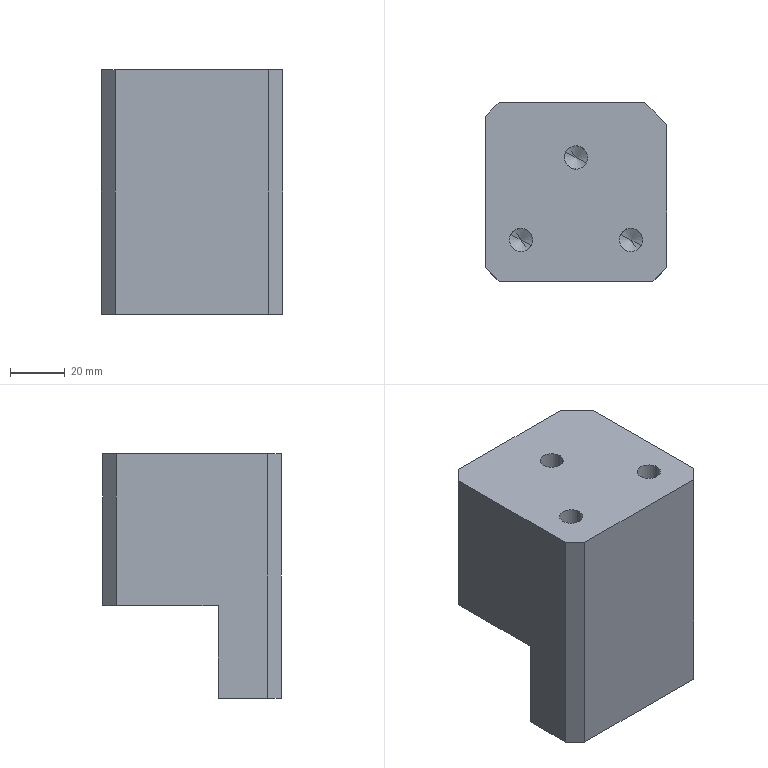Part | CATIA | 1 solid | 40 faces | box 66 x 65 x 89 mm | volume 271119 mm3 | cone 14 | cylinder 14 | plane 12 | commonest cylinder face diameters 8.5 x12 10 x2
STEP:
#1=CARTESIAN_POINT('',(63.,-90.,84.));
#2=VERTEX_POINT('',#1);
#3=CARTESIAN_POINT('',(58.,-85.,84.));
#4=VERTEX_POINT('',#3);
#5=CARTESIAN_POINT('',(60.5,-87.5,84.));
#6=DIRECTION('',(-0.7071,0.7071,0.));
#7=VECTOR('',#6,1.);
#8=LINE('',#5,#7);
#9=EDGE_CURVE('',#2,#4,#8,.T.);
#10=ORIENTED_EDGE('',*,*,#9,.T.);
#11=CARTESIAN_POINT('',(58.,-85.,-5.));
#12=VERTEX_POINT('',#11);
#13=CARTESIAN_POINT('',(58.,-85.,39.5));
#14=DIRECTION('',(0.,0.,1.));
#15=VECTOR('',#14,1.);
#16=LINE('',#13,#15);
#17=EDGE_CURVE('',#12,#4,#16,.T.);
#18=ORIENTED_EDGE('',*,*,#17,.F.);
#19=CARTESIAN_POINT('',(63.,-90.,-5.));
#20=VERTEX_POINT('',#19);
#21=CARTESIAN_POINT('',(60.5,-87.5,-5.));
#22=DIRECTION('',(-0.7071,0.7071,0.));
#23=VECTOR('',#22,1.);
#24=LINE('',#21,#23);
#25=EDGE_CURVE('',#12,#20,#24,.F.);
#26=ORIENTED_EDGE('',*,*,#25,.T.);
#27=CARTESIAN_POINT('',(63.,-90.,39.5));
#28=DIRECTION('',(0.,0.,1.));
#29=VECTOR('',#28,1.);
#30=LINE('',#27,#29);
#31=EDGE_CURVE('',#20,#2,#30,.T.);
#32=ORIENTED_EDGE('',*,*,#31,.T.);
#33=EDGE_LOOP('',(#10,#18,#26,#32));
#34=FACE_OUTER_BOUND('',#33,.T.);
#35=CARTESIAN_POINT('',(63.,-90.,-22.8));
#36=DIRECTION('',(-0.7071,-0.7071,0.));
#37=DIRECTION('',(0.,0.,1.));
#38=AXIS2_PLACEMENT_3D('',#35,#36,#37);
#39=PLANE('',#38);
#40=ADVANCED_FACE('',(#34),#39,.T.);
#41=CARTESIAN_POINT('',(119.,-90.,84.));
#42=VERTEX_POINT('',#41);
#43=CARTESIAN_POINT('',(91.,-90.,84.));
#44=DIRECTION('',(1.,0.,0.));
#45=VECTOR('',#44,1.);
#46=LINE('',#43,#45);
#47=EDGE_CURVE('',#2,#42,#46,.T.);
#48=ORIENTED_EDGE('',*,*,#47,.F.);
#49=ORIENTED_EDGE('',*,*,#31,.F.);
#50=CARTESIAN_POINT('',(119.,-90.,-5.));
#51=VERTEX_POINT('',#50);
#52=CARTESIAN_POINT('',(91.,-90.,-5.));
#53=DIRECTION('',(1.,0.,0.));
#54=VECTOR('',#53,1.);
#55=LINE('',#52,#54);
#56=EDGE_CURVE('',#51,#20,#55,.F.);
#57=ORIENTED_EDGE('',*,*,#56,.F.);
#58=CARTESIAN_POINT('',(119.,-90.,39.5));
#59=DIRECTION('',(0.,0.,-1.));
#60=VECTOR('',#59,1.);
#61=LINE('',#58,#60);
#62=EDGE_CURVE('',#51,#42,#61,.F.);
#63=ORIENTED_EDGE('',*,*,#62,.T.);
#64=EDGE_LOOP('',(#48,#49,#57,#63));
#65=FACE_OUTER_BOUND('',#64,.T.);
#66=CARTESIAN_POINT('',(58.,-90.,0.));
#67=DIRECTION('',(0.,-1.,0.));
#68=DIRECTION('',(1.,0.,0.));
#69=AXIS2_PLACEMENT_3D('',#66,#67,#68);
#70=PLANE('',#69);
#71=ADVANCED_FACE('',(#65),#70,.T.);
#72=CARTESIAN_POINT('',(124.,-85.,84.));
#73=VERTEX_POINT('',#72);
#74=CARTESIAN_POINT('',(121.5,-87.5,84.));
#75=DIRECTION('',(0.7071,0.7071,0.));
#76=VECTOR('',#75,1.);
#77=LINE('',#74,#76);
#78=EDGE_CURVE('',#73,#42,#77,.F.);
#79=ORIENTED_EDGE('',*,*,#78,.T.);
#80=ORIENTED_EDGE('',*,*,#62,.F.);
#81=CARTESIAN_POINT('',(124.,-85.,-5.));
#82=VERTEX_POINT('',#81);
#83=CARTESIAN_POINT('',(121.5,-87.5,-5.));
#84=DIRECTION('',(0.7071,0.7071,0.));
#85=VECTOR('',#84,1.);
#86=LINE('',#83,#85);
#87=EDGE_CURVE('',#51,#82,#86,.T.);
#88=ORIENTED_EDGE('',*,*,#87,.T.);
#89=CARTESIAN_POINT('',(124.,-85.,39.5));
#90=DIRECTION('',(0.,0.,-1.));
#91=VECTOR('',#90,1.);
#92=LINE('',#89,#91);
#93=EDGE_CURVE('',#82,#73,#92,.F.);
#94=ORIENTED_EDGE('',*,*,#93,.T.);
#95=EDGE_LOOP('',(#79,#80,#88,#94));
#96=FACE_OUTER_BOUND('',#95,.T.);
#97=CARTESIAN_POINT('',(119.,-90.,101.8));
#98=DIRECTION('',(0.7071,-0.7071,0.));
#99=DIRECTION('',(0.,0.,-1.));
#100=AXIS2_PLACEMENT_3D('',#97,#98,#99);
#101=PLANE('',#100);
#102=ADVANCED_FACE('',(#96),#101,.T.);
#103=CARTESIAN_POINT('',(116.,-25.,84.));
#104=VERTEX_POINT('',#103);
#105=CARTESIAN_POINT('',(63.,-25.,84.));
#106=VERTEX_POINT('',#105);
#107=CARTESIAN_POINT('',(89.5,-25.,84.));
#108=DIRECTION('',(-1.,0.,0.));
#109=VECTOR('',#108,1.);
#110=LINE('',#107,#109);
#111=EDGE_CURVE('',#104,#106,#110,.T.);
#112=ORIENTED_EDGE('',*,*,#111,.T.);
#113=CARTESIAN_POINT('',(58.,-30.,84.));
#114=VERTEX_POINT('',#113);
#115=CARTESIAN_POINT('',(60.5,-27.5,84.));
#116=DIRECTION('',(0.7071,0.7071,0.));
#117=VECTOR('',#116,1.);
#118=LINE('',#115,#117);
#119=EDGE_CURVE('',#114,#106,#118,.T.);
#120=ORIENTED_EDGE('',*,*,#119,.F.);
#121=CARTESIAN_POINT('',(58.,-57.5,84.));
#122=DIRECTION('',(0.,1.,0.));
#123=VECTOR('',#122,1.);
#124=LINE('',#121,#123);
#125=EDGE_CURVE('',#4,#114,#124,.T.);
#126=ORIENTED_EDGE('',*,*,#125,.F.);
#127=ORIENTED_EDGE('',*,*,#9,.F.);
#128=ORIENTED_EDGE('',*,*,#47,.T.);
#129=ORIENTED_EDGE('',*,*,#78,.F.);
#130=CARTESIAN_POINT('',(124.,-33.,84.));
#131=VERTEX_POINT('',#130);
#132=CARTESIAN_POINT('',(124.,-59.,84.));
#133=DIRECTION('',(0.,-1.,0.));
#134=VECTOR('',#133,1.);
#135=LINE('',#132,#134);
#136=EDGE_CURVE('',#131,#73,#135,.T.);
#137=ORIENTED_EDGE('',*,*,#136,.F.);
#138=CARTESIAN_POINT('',(120.,-29.,84.));
#139=DIRECTION('',(0.7071,-0.7071,0.));
#140=VECTOR('',#139,1.);
#141=LINE('',#138,#140);
#142=EDGE_CURVE('',#104,#131,#141,.T.);
#143=ORIENTED_EDGE('',*,*,#142,.F.);
#144=EDGE_LOOP('',(#112,#120,#126,#127,#128,#129,#137,#143));
#145=FACE_OUTER_BOUND('',#144,.T.);
#146=CARTESIAN_POINT('',(114.73,-77.038,84.));
#147=VERTEX_POINT('',#146);
#148=CARTESIAN_POINT('',(107.27,-72.962,84.));
#149=VERTEX_POINT('',#148);
#150=CARTESIAN_POINT('',(111.,-75.,84.));
#151=DIRECTION('',(0.,0.,1.));
#152=AXIS2_PLACEMENT_3D('',#150,#151,$);
#153=CIRCLE('',#152,4.25);
#154=EDGE_CURVE('',#147,#149,#153,.T.);
#155=ORIENTED_EDGE('',*,*,#154,.F.);
#156=CARTESIAN_POINT('',(111.,-75.,84.));
#157=DIRECTION('',(0.,0.,1.));
#158=AXIS2_PLACEMENT_3D('',#156,#157,$);
#159=CIRCLE('',#158,4.25);
#160=EDGE_CURVE('',#149,#147,#159,.T.);
#161=ORIENTED_EDGE('',*,*,#160,.F.);
#162=EDGE_LOOP('',(#155,#161));
#163=FACE_BOUND('',#162,.T.);
#164=CARTESIAN_POINT('',(74.73,-77.038,84.));
#165=VERTEX_POINT('',#164);
#166=CARTESIAN_POINT('',(67.27,-72.962,84.));
#167=VERTEX_POINT('',#166);
#168=CARTESIAN_POINT('',(71.,-75.,84.));
#169=DIRECTION('',(0.,0.,1.));
#170=AXIS2_PLACEMENT_3D('',#168,#169,$);
#171=CIRCLE('',#170,4.25);
#172=EDGE_CURVE('',#165,#167,#171,.T.);
#173=ORIENTED_EDGE('',*,*,#172,.F.);
#174=CARTESIAN_POINT('',(71.,-75.,84.));
#175=DIRECTION('',(0.,0.,1.));
#176=AXIS2_PLACEMENT_3D('',#174,#175,$);
#177=CIRCLE('',#176,4.25);
#178=EDGE_CURVE('',#167,#165,#177,.T.);
#179=ORIENTED_EDGE('',*,*,#178,.F.);
#180=EDGE_LOOP('',(#173,#179));
#181=FACE_BOUND('',#180,.T.);
#182=CARTESIAN_POINT('',(94.73,-47.038,84.));
#183=VERTEX_POINT('',#182);
#184=CARTESIAN_POINT('',(87.27,-42.962,84.));
#185=VERTEX_POINT('',#184);
#186=CARTESIAN_POINT('',(91.,-45.,84.));
#187=DIRECTION('',(0.,0.,1.));
#188=AXIS2_PLACEMENT_3D('',#186,#187,$);
#189=CIRCLE('',#188,4.25);
#190=EDGE_CURVE('',#183,#185,#189,.T.);
#191=ORIENTED_EDGE('',*,*,#190,.F.);
#192=CARTESIAN_POINT('',(91.,-45.,84.));
#193=DIRECTION('',(0.,0.,1.));
#194=AXIS2_PLACEMENT_3D('',#192,#193,$);
#195=CIRCLE('',#194,4.25);
#196=EDGE_CURVE('',#185,#183,#195,.T.);
#197=ORIENTED_EDGE('',*,*,#196,.F.);
#198=EDGE_LOOP('',(#191,#197));
#199=FACE_BOUND('',#198,.T.);
#200=CARTESIAN_POINT('',(0.,0.,84.));
#201=DIRECTION('',(0.,0.,1.));
#202=DIRECTION('',(1.,0.,0.));
#203=AXIS2_PLACEMENT_3D('',#200,#201,#202);
#204=PLANE('',#203);
#205=ADVANCED_FACE('',(#145,#163,#181,#199),#204,.T.);
#206=CARTESIAN_POINT('',(91.,-45.,51.546));
#207=VERTEX_POINT('',#206);
#208=CARTESIAN_POINT('',(94.73,-47.038,54.));
#209=VERTEX_POINT('',#208);
#210=CARTESIAN_POINT('',(92.865,-46.019,52.773));
#211=DIRECTION('',(0.76,-0.4152,0.5));
#212=VECTOR('',#211,1.);
#213=LINE('',#210,#212);
#214=EDGE_CURVE('',#207,#209,#213,.T.);
#215=ORIENTED_EDGE('',*,*,#214,.T.);
#216=CARTESIAN_POINT('',(87.27,-42.962,54.));
#217=VERTEX_POINT('',#216);
#218=CARTESIAN_POINT('',(91.,-45.,54.));
#219=DIRECTION('',(0.,0.,1.));
#220=AXIS2_PLACEMENT_3D('',#218,#219,$);
#221=CIRCLE('',#220,4.25);
#222=EDGE_CURVE('',#217,#209,#221,.F.);
#223=ORIENTED_EDGE('',*,*,#222,.F.);
#224=CARTESIAN_POINT('',(89.135,-43.981,52.773));
#225=DIRECTION('',(-0.76,0.4152,0.5));
#226=VECTOR('',#225,1.);
#227=LINE('',#224,#226);
#228=EDGE_CURVE('',#207,#217,#227,.T.);
#229=ORIENTED_EDGE('',*,*,#228,.F.);
#230=EDGE_LOOP('',(#215,#223,#229));
#231=FACE_OUTER_BOUND('',#230,.T.);
#232=CARTESIAN_POINT('',(91.,-45.,51.546));
#233=DIRECTION('',(0.,0.,1.));
#234=DIRECTION('',(0.8776,-0.4794,0.));
#235=AXIS2_PLACEMENT_3D('',#232,#233,#234);
#236=CONICAL_SURFACE('',#235,0.,1.047);
#237=ADVANCED_FACE('',(#231),#236,.F.);
#238=ORIENTED_EDGE('',*,*,#190,.T.);
#239=CARTESIAN_POINT('',(87.27,-42.962,69.2));
#240=DIRECTION('',(0.,0.,-1.));
#241=VECTOR('',#240,1.);
#242=LINE('',#239,#241);
#243=EDGE_CURVE('',#217,#185,#242,.F.);
#244=ORIENTED_EDGE('',*,*,#243,.F.);
#245=ORIENTED_EDGE('',*,*,#222,.T.);
#246=CARTESIAN_POINT('',(94.73,-47.038,69.2));
#247=DIRECTION('',(0.,0.,-1.));
#248=VECTOR('',#247,1.);
#249=LINE('',#246,#248);
#250=EDGE_CURVE('',#209,#183,#249,.F.);
#251=ORIENTED_EDGE('',*,*,#250,.T.);
#252=EDGE_LOOP('',(#238,#244,#245,#251));
#253=FACE_OUTER_BOUND('',#252,.T.);
#254=CARTESIAN_POINT('',(91.,-45.,83.9));
#255=DIRECTION('',(0.,0.,-1.));
#256=DIRECTION('',(0.8776,-0.4794,0.));
#257=AXIS2_PLACEMENT_3D('',#254,#255,#256);
#258=CYLINDRICAL_SURFACE('',#257,4.25);
#259=ADVANCED_FACE('',(#253),#258,.F.);
#260=CARTESIAN_POINT('',(71.,-75.,51.546));
#261=VERTEX_POINT('',#260);
#262=CARTESIAN_POINT('',(67.27,-72.962,54.));
#263=VERTEX_POINT('',#262);
#264=CARTESIAN_POINT('',(69.135,-73.981,52.773));
#265=DIRECTION('',(-0.76,0.4152,0.5));
#266=VECTOR('',#265,1.);
#267=LINE('',#264,#266);
#268=EDGE_CURVE('',#261,#263,#267,.T.);
#269=ORIENTED_EDGE('',*,*,#268,.T.);
#270=CARTESIAN_POINT('',(74.73,-77.038,54.));
#271=VERTEX_POINT('',#270);
#272=CARTESIAN_POINT('',(71.,-75.,54.));
#273=DIRECTION('',(0.,0.,1.));
#274=AXIS2_PLACEMENT_3D('',#272,#273,$);
#275=CIRCLE('',#274,4.25);
#276=EDGE_CURVE('',#271,#263,#275,.F.);
#277=ORIENTED_EDGE('',*,*,#276,.F.);
#278=CARTESIAN_POINT('',(72.865,-76.019,52.773));
#279=DIRECTION('',(0.76,-0.4152,0.5));
#280=VECTOR('',#279,1.);
#281=LINE('',#278,#280);
#282=EDGE_CURVE('',#261,#271,#281,.T.);
#283=ORIENTED_EDGE('',*,*,#282,.F.);
#284=EDGE_LOOP('',(#269,#277,#283));
#285=FACE_OUTER_BOUND('',#284,.T.);
#286=CARTESIAN_POINT('',(71.,-75.,51.546));
#287=DIRECTION('',(0.,0.,1.));
#288=DIRECTION('',(0.8776,-0.4794,0.));
#289=AXIS2_PLACEMENT_3D('',#286,#287,#288);
#290=CONICAL_SURFACE('',#289,0.,1.047);
#291=ADVANCED_FACE('',(#285),#290,.F.);
#292=ORIENTED_EDGE('',*,*,#282,.T.);
#293=CARTESIAN_POINT('',(71.,-75.,54.));
#294=DIRECTION('',(0.,0.,1.));
#295=AXIS2_PLACEMENT_3D('',#293,#294,$);
#296=CIRCLE('',#295,4.25);
#297=EDGE_CURVE('',#263,#271,#296,.F.);
#298=ORIENTED_EDGE('',*,*,#297,.F.);
#299=ORIENTED_EDGE('',*,*,#268,.F.);
#300=EDGE_LOOP('',(#292,#298,#299));
#301=FACE_OUTER_BOUND('',#300,.T.);
#302=ADVANCED_FACE('',(#301),#290,.F.);
#303=ORIENTED_EDGE('',*,*,#178,.T.);
#304=CARTESIAN_POINT('',(74.73,-77.038,69.2));
#305=DIRECTION('',(0.,0.,-1.));
#306=VECTOR('',#305,1.);
#307=LINE('',#304,#306);
#308=EDGE_CURVE('',#271,#165,#307,.F.);
#309=ORIENTED_EDGE('',*,*,#308,.F.);
#310=ORIENTED_EDGE('',*,*,#276,.T.);
#311=CARTESIAN_POINT('',(67.27,-72.962,69.2));
#312=DIRECTION('',(0.,0.,-1.));
#313=VECTOR('',#312,1.);
#314=LINE('',#311,#313);
#315=EDGE_CURVE('',#263,#167,#314,.F.);
#316=ORIENTED_EDGE('',*,*,#315,.T.);
#317=EDGE_LOOP('',(#303,#309,#310,#316));
#318=FACE_OUTER_BOUND('',#317,.T.);
#319=CARTESIAN_POINT('',(71.,-75.,83.9));
#320=DIRECTION('',(0.,0.,-1.));
#321=DIRECTION('',(0.8776,-0.4794,0.));
#322=AXIS2_PLACEMENT_3D('',#319,#320,#321);
#323=CYLINDRICAL_SURFACE('',#322,4.25);
#324=ADVANCED_FACE('',(#318),#323,.F.);
#325=ORIENTED_EDGE('',*,*,#172,.T.);
#326=ORIENTED_EDGE('',*,*,#315,.F.);
#327=ORIENTED_EDGE('',*,*,#297,.T.);
#328=ORIENTED_EDGE('',*,*,#308,.T.);
#329=EDGE_LOOP('',(#325,#326,#327,#328));
#330=FACE_OUTER_BOUND('',#329,.T.);
#331=ADVANCED_FACE('',(#330),#323,.F.);
#332=CARTESIAN_POINT('',(111.,-75.,51.546));
#333=VERTEX_POINT('',#332);
#334=CARTESIAN_POINT('',(107.27,-72.962,54.));
#335=VERTEX_POINT('',#334);
#336=CARTESIAN_POINT('',(109.135,-73.981,52.773));
#337=DIRECTION('',(-0.76,0.4152,0.5));
#338=VECTOR('',#337,1.);
#339=LINE('',#336,#338);
#340=EDGE_CURVE('',#333,#335,#339,.T.);
#341=ORIENTED_EDGE('',*,*,#340,.T.);
#342=CARTESIAN_POINT('',(114.73,-77.038,54.));
#343=VERTEX_POINT('',#342);
#344=CARTESIAN_POINT('',(111.,-75.,54.));
#345=DIRECTION('',(0.,0.,1.));
#346=AXIS2_PLACEMENT_3D('',#344,#345,$);
#347=CIRCLE('',#346,4.25);
#348=EDGE_CURVE('',#343,#335,#347,.F.);
#349=ORIENTED_EDGE('',*,*,#348,.F.);
#350=CARTESIAN_POINT('',(112.865,-76.019,52.773));
#351=DIRECTION('',(0.76,-0.4152,0.5));
#352=VECTOR('',#351,1.);
#353=LINE('',#350,#352);
#354=EDGE_CURVE('',#333,#343,#353,.T.);
#355=ORIENTED_EDGE('',*,*,#354,.F.);
#356=EDGE_LOOP('',(#341,#349,#355));
#357=FACE_OUTER_BOUND('',#356,.T.);
#358=CARTESIAN_POINT('',(111.,-75.,51.546));
#359=DIRECTION('',(0.,0.,1.));
#360=DIRECTION('',(0.8776,-0.4794,0.));
#361=AXIS2_PLACEMENT_3D('',#358,#359,#360);
#362=CONICAL_SURFACE('',#361,0.,1.047);
#363=ADVANCED_FACE('',(#357),#362,.F.);
#364=ORIENTED_EDGE('',*,*,#354,.T.);
#365=CARTESIAN_POINT('',(111.,-75.,54.));
#366=DIRECTION('',(0.,0.,1.));
#367=AXIS2_PLACEMENT_3D('',#365,#366,$);
#368=CIRCLE('',#367,4.25);
#369=EDGE_CURVE('',#335,#343,#368,.F.);
#370=ORIENTED_EDGE('',*,*,#369,.F.);
#371=ORIENTED_EDGE('',*,*,#340,.F.);
#372=EDGE_LOOP('',(#364,#370,#371));
#373=FACE_OUTER_BOUND('',#372,.T.);
#374=ADVANCED_FACE('',(#373),#362,.F.);
#375=ORIENTED_EDGE('',*,*,#160,.T.);
#376=CARTESIAN_POINT('',(114.73,-77.038,69.2));
#377=DIRECTION('',(0.,0.,-1.));
#378=VECTOR('',#377,1.);
#379=LINE('',#376,#378);
#380=EDGE_CURVE('',#343,#147,#379,.F.);
#381=ORIENTED_EDGE('',*,*,#380,.F.);
#382=ORIENTED_EDGE('',*,*,#348,.T.);
#383=CARTESIAN_POINT('',(107.27,-72.962,69.2));
#384=DIRECTION('',(0.,0.,-1.));
#385=VECTOR('',#384,1.);
#386=LINE('',#383,#385);
#387=EDGE_CURVE('',#335,#149,#386,.F.);
#388=ORIENTED_EDGE('',*,*,#387,.T.);
#389=EDGE_LOOP('',(#375,#381,#382,#388));
#390=FACE_OUTER_BOUND('',#389,.T.);
#391=CARTESIAN_POINT('',(111.,-75.,83.9));
#392=DIRECTION('',(0.,0.,-1.));
#393=DIRECTION('',(0.8776,-0.4794,0.));
#394=AXIS2_PLACEMENT_3D('',#391,#392,#393);
#395=CYLINDRICAL_SURFACE('',#394,4.25);
#396=ADVANCED_FACE('',(#390),#395,.F.);
#397=ORIENTED_EDGE('',*,*,#154,.T.);
#398=ORIENTED_EDGE('',*,*,#387,.F.);
#399=ORIENTED_EDGE('',*,*,#369,.T.);
#400=ORIENTED_EDGE('',*,*,#380,.T.);
#401=EDGE_LOOP('',(#397,#398,#399,#400));
#402=FACE_OUTER_BOUND('',#401,.T.);
#403=ADVANCED_FACE('',(#402),#395,.F.);
#404=CARTESIAN_POINT('',(89.608,-49.015,54.));
#405=VERTEX_POINT('',#404);
#406=CARTESIAN_POINT('',(91.477,-49.223,54.));
#407=VERTEX_POINT('',#406);
#408=CARTESIAN_POINT('',(89.608,-49.015,54.));
#409=CARTESIAN_POINT('',(89.949,-49.134,54.084));
#410=CARTESIAN_POINT('',(90.323,-49.224,54.138));
#411=CARTESIAN_POINT('',(90.733,-49.27,54.138));
#412=CARTESIAN_POINT('',(91.118,-49.264,54.084));
#413=CARTESIAN_POINT('',(91.477,-49.223,54.));
#414=B_SPLINE_CURVE_WITH_KNOTS('',5,(#408,#409,#410,#411,#412,#413),.UNSPECIFIED.,.F.,.U.,(6,6),(0.,2.197),.UNSPECIFIED.);
#415=EDGE_CURVE('',#405,#407,#414,.T.);
#416=ORIENTED_EDGE('',*,*,#415,.F.);
#417=CARTESIAN_POINT('',(91.,-45.,54.));
#418=DIRECTION('',(0.,0.,-1.));
#419=AXIS2_PLACEMENT_3D('',#417,#418,$);
#420=CIRCLE('',#419,4.25);
#421=EDGE_CURVE('',#405,#217,#420,.T.);
#422=ORIENTED_EDGE('',*,*,#421,.T.);
#423=ORIENTED_EDGE('',*,*,#243,.T.);
#424=ORIENTED_EDGE('',*,*,#196,.T.);
#425=ORIENTED_EDGE('',*,*,#250,.F.);
#426=CARTESIAN_POINT('',(91.,-45.,54.));
#427=DIRECTION('',(0.,0.,-1.));
#428=AXIS2_PLACEMENT_3D('',#426,#427,$);
#429=CIRCLE('',#428,4.25);
#430=EDGE_CURVE('',#209,#407,#429,.T.);
#431=ORIENTED_EDGE('',*,*,#430,.T.);
#432=EDGE_LOOP('',(#416,#422,#423,#424,#425,#431));
#433=FACE_OUTER_BOUND('',#432,.T.);
#434=ADVANCED_FACE('',(#433),#258,.F.);
#435=CARTESIAN_POINT('',(91.477,-49.223,54.));
#436=CARTESIAN_POINT('',(91.132,-49.117,53.916));
#437=CARTESIAN_POINT('',(90.758,-49.034,53.862));
#438=CARTESIAN_POINT('',(90.351,-48.989,53.862));
#439=CARTESIAN_POINT('',(89.967,-48.987,53.916));
#440=CARTESIAN_POINT('',(89.608,-49.015,54.));
#441=B_SPLINE_CURVE_WITH_KNOTS('',5,(#435,#436,#437,#438,#439,#440),.UNSPECIFIED.,.F.,.U.,(6,6),(0.,2.194),.UNSPECIFIED.);
#442=EDGE_CURVE('',#407,#405,#441,.T.);
#443=ORIENTED_EDGE('',*,*,#442,.F.);
#444=ORIENTED_EDGE('',*,*,#430,.F.);
#445=ORIENTED_EDGE('',*,*,#214,.F.);
#446=ORIENTED_EDGE('',*,*,#228,.T.);
#447=ORIENTED_EDGE('',*,*,#421,.F.);
#448=EDGE_LOOP('',(#443,#444,#445,#446,#447));
#449=FACE_OUTER_BOUND('',#448,.T.);
#450=ADVANCED_FACE('',(#449),#236,.F.);
#451=CARTESIAN_POINT('',(116.,-25.,28.7));
#452=VERTEX_POINT('',#451);
#453=CARTESIAN_POINT('',(116.,-25.,39.5));
#454=DIRECTION('',(0.,0.,1.));
#455=VECTOR('',#454,1.);
#456=LINE('',#453,#455);
#457=EDGE_CURVE('',#452,#104,#456,.T.);
#458=ORIENTED_EDGE('',*,*,#457,.T.);
#459=ORIENTED_EDGE('',*,*,#142,.T.);
#460=CARTESIAN_POINT('',(124.,-33.,28.7));
#461=VERTEX_POINT('',#460);
#462=CARTESIAN_POINT('',(124.,-33.,39.5));
#463=DIRECTION('',(0.,0.,1.));
#464=VECTOR('',#463,1.);
#465=LINE('',#462,#464);
#466=EDGE_CURVE('',#461,#131,#465,.T.);
#467=ORIENTED_EDGE('',*,*,#466,.F.);
#468=CARTESIAN_POINT('',(120.,-29.,28.7));
#469=DIRECTION('',(0.7071,-0.7071,0.));
#470=VECTOR('',#469,1.);
#471=LINE('',#468,#470);
#472=EDGE_CURVE('',#461,#452,#471,.F.);
#473=ORIENTED_EDGE('',*,*,#472,.T.);
#474=EDGE_LOOP('',(#458,#459,#467,#473));
#475=FACE_OUTER_BOUND('',#474,.T.);
#476=CARTESIAN_POINT('',(116.,-25.,-22.8));
#477=DIRECTION('',(0.7071,0.7071,0.));
#478=DIRECTION('',(0.,0.,1.));
#479=AXIS2_PLACEMENT_3D('',#476,#477,#478);
#480=PLANE('',#479);
#481=ADVANCED_FACE('',(#475),#480,.T.);
#482=CARTESIAN_POINT('',(124.,-67.,28.7));
#483=VERTEX_POINT('',#482);
#484=CARTESIAN_POINT('',(124.,-67.,-5.));
#485=VERTEX_POINT('',#484);
#486=CARTESIAN_POINT('',(124.,-67.,11.85));
#487=DIRECTION('',(0.,0.,-1.));
#488=VECTOR('',#487,1.);
#489=LINE('',#486,#488);
#490=EDGE_CURVE('',#483,#485,#489,.T.);
#491=ORIENTED_EDGE('',*,*,#490,.F.);
#492=CARTESIAN_POINT('',(124.,-50.,28.7));
#493=DIRECTION('',(0.,1.,0.));
#494=VECTOR('',#493,1.);
#495=LINE('',#492,#494);
#496=EDGE_CURVE('',#483,#461,#495,.T.);
#497=ORIENTED_EDGE('',*,*,#496,.T.);
#498=ORIENTED_EDGE('',*,*,#466,.T.);
#499=ORIENTED_EDGE('',*,*,#136,.T.);
#500=ORIENTED_EDGE('',*,*,#93,.F.);
#501=CARTESIAN_POINT('',(124.,-76.,-5.));
#502=DIRECTION('',(0.,-1.,0.));
#503=VECTOR('',#502,1.);
#504=LINE('',#501,#503);
#505=EDGE_CURVE('',#485,#82,#504,.T.);
#506=ORIENTED_EDGE('',*,*,#505,.F.);
#507=EDGE_LOOP('',(#491,#497,#498,#499,#500,#506));
#508=FACE_OUTER_BOUND('',#507,.T.);
#509=CARTESIAN_POINT('',(124.,-25.,0.));
#510=DIRECTION('',(-1.,0.,0.));
#511=DIRECTION('',(0.,-1.,0.));
#512=AXIS2_PLACEMENT_3D('',#509,#510,#511);
#513=PLANE('',#512);
#514=ADVANCED_FACE('',(#508),#513,.F.);
#515=CARTESIAN_POINT('',(63.,-25.,28.7));
#516=VERTEX_POINT('',#515);
#517=CARTESIAN_POINT('',(63.,-25.,56.35));
#518=DIRECTION('',(0.,0.,-1.));
#519=VECTOR('',#518,1.);
#520=LINE('',#517,#519);
#521=EDGE_CURVE('',#516,#106,#520,.F.);
#522=ORIENTED_EDGE('',*,*,#521,.T.);
#523=ORIENTED_EDGE('',*,*,#111,.F.);
#524=ORIENTED_EDGE('',*,*,#457,.F.);
#525=CARTESIAN_POINT('',(89.5,-25.,28.7));
#526=DIRECTION('',(-1.,0.,0.));
#527=VECTOR('',#526,1.);
#528=LINE('',#525,#527);
#529=EDGE_CURVE('',#452,#516,#528,.T.);
#530=ORIENTED_EDGE('',*,*,#529,.T.);
#531=EDGE_LOOP('',(#522,#523,#524,#530));
#532=FACE_OUTER_BOUND('',#531,.T.);
#533=CARTESIAN_POINT('',(124.,-25.,0.));
#534=DIRECTION('',(0.,1.,0.));
#535=DIRECTION('',(-1.,0.,0.));
#536=AXIS2_PLACEMENT_3D('',#533,#534,#535);
#537=PLANE('',#536);
#538=ADVANCED_FACE('',(#532),#537,.T.);
#539=CARTESIAN_POINT('',(58.,-30.,28.7));
#540=VERTEX_POINT('',#539);
#541=CARTESIAN_POINT('',(58.,-30.,39.5));
#542=DIRECTION('',(0.,0.,-1.));
#543=VECTOR('',#542,1.);
#544=LINE('',#541,#543);
#545=EDGE_CURVE('',#540,#114,#544,.F.);
#546=ORIENTED_EDGE('',*,*,#545,.T.);
#547=ORIENTED_EDGE('',*,*,#119,.T.);
#548=ORIENTED_EDGE('',*,*,#521,.F.);
#549=CARTESIAN_POINT('',(60.5,-27.5,28.7));
#550=DIRECTION('',(-0.7071,-0.7071,0.));
#551=VECTOR('',#550,1.);
#552=LINE('',#549,#551);
#553=EDGE_CURVE('',#540,#516,#552,.F.);
#554=ORIENTED_EDGE('',*,*,#553,.F.);
#555=EDGE_LOOP('',(#546,#547,#548,#554));
#556=FACE_OUTER_BOUND('',#555,.T.);
#557=CARTESIAN_POINT('',(63.,-25.,101.8));
#558=DIRECTION('',(-0.7071,0.7071,0.));
#559=DIRECTION('',(0.,0.,-1.));
#560=AXIS2_PLACEMENT_3D('',#557,#558,#559);
#561=PLANE('',#560);
#562=ADVANCED_FACE('',(#556),#561,.T.);
#563=CARTESIAN_POINT('',(58.,-67.,28.7));
#564=VERTEX_POINT('',#563);
#565=CARTESIAN_POINT('',(58.,-48.5,28.7));
#566=DIRECTION('',(0.,1.,0.));
#567=VECTOR('',#566,1.);
#568=LINE('',#565,#567);
#569=EDGE_CURVE('',#564,#540,#568,.T.);
#570=ORIENTED_EDGE('',*,*,#569,.F.);
#571=CARTESIAN_POINT('',(58.,-67.,-5.));
#572=VERTEX_POINT('',#571);
#573=CARTESIAN_POINT('',(58.,-67.,11.85));
#574=DIRECTION('',(0.,0.,-1.));
#575=VECTOR('',#574,1.);
#576=LINE('',#573,#575);
#577=EDGE_CURVE('',#564,#572,#576,.T.);
#578=ORIENTED_EDGE('',*,*,#577,.T.);
#579=CARTESIAN_POINT('',(58.,-76.,-5.));
#580=DIRECTION('',(0.,1.,0.));
#581=VECTOR('',#580,1.);
#582=LINE('',#579,#581);
#583=EDGE_CURVE('',#12,#572,#582,.T.);
#584=ORIENTED_EDGE('',*,*,#583,.F.);
#585=ORIENTED_EDGE('',*,*,#17,.T.);
#586=ORIENTED_EDGE('',*,*,#125,.T.);
#587=ORIENTED_EDGE('',*,*,#545,.F.);
#588=EDGE_LOOP('',(#570,#578,#584,#585,#586,#587));
#589=FACE_OUTER_BOUND('',#588,.T.);
#590=CARTESIAN_POINT('',(58.,-90.,0.));
#591=DIRECTION('',(1.,0.,0.));
#592=DIRECTION('',(0.,1.,0.));
#593=AXIS2_PLACEMENT_3D('',#590,#591,#592);
#594=PLANE('',#593);
#595=ADVANCED_FACE('',(#589),#594,.F.);
#596=CARTESIAN_POINT('',(71.,-54.,61.454));
#597=VERTEX_POINT('',#596);
#598=CARTESIAN_POINT('',(67.27,-56.038,59.));
#599=VERTEX_POINT('',#598);
#600=CARTESIAN_POINT('',(69.135,-55.019,60.227));
#601=DIRECTION('',(-0.76,-0.4152,-0.5));
#602=VECTOR('',#601,1.);
#603=LINE('',#600,#602);
#604=EDGE_CURVE('',#597,#599,#603,.T.);
#605=ORIENTED_EDGE('',*,*,#604,.T.);
#606=CARTESIAN_POINT('',(74.73,-51.962,59.));
#607=VERTEX_POINT('',#606);
#608=CARTESIAN_POINT('',(71.,-54.,59.));
#609=DIRECTION('',(0.,0.,-1.));
#610=AXIS2_PLACEMENT_3D('',#608,#609,$);
#611=CIRCLE('',#610,4.25);
#612=EDGE_CURVE('',#607,#599,#611,.F.);
#613=ORIENTED_EDGE('',*,*,#612,.F.);
#614=CARTESIAN_POINT('',(72.865,-52.981,60.227));
#615=DIRECTION('',(0.76,0.4152,-0.5));
#616=VECTOR('',#615,1.);
#617=LINE('',#614,#616);
#618=EDGE_CURVE('',#597,#607,#617,.T.);
#619=ORIENTED_EDGE('',*,*,#618,.F.);
#620=EDGE_LOOP('',(#605,#613,#619));
#621=FACE_OUTER_BOUND('',#620,.T.);
#622=CARTESIAN_POINT('',(71.,-54.,61.454));
#623=DIRECTION('',(0.,0.,-1.));
#624=DIRECTION('',(0.8776,0.4794,0.));
#625=AXIS2_PLACEMENT_3D('',#622,#623,#624);
#626=CONICAL_SURFACE('',#625,0.,1.047);
#627=ADVANCED_FACE('',(#621),#626,.F.);
#628=ORIENTED_EDGE('',*,*,#618,.T.);
#629=CARTESIAN_POINT('',(71.,-54.,59.));
#630=DIRECTION('',(0.,0.,-1.));
#631=AXIS2_PLACEMENT_3D('',#629,#630,$);
#632=CIRCLE('',#631,4.25);
#633=EDGE_CURVE('',#599,#607,#632,.F.);
#634=ORIENTED_EDGE('',*,*,#633,.F.);
#635=ORIENTED_EDGE('',*,*,#604,.F.);
#636=EDGE_LOOP('',(#628,#634,#635));
#637=FACE_OUTER_BOUND('',#636,.T.);
#638=ADVANCED_FACE('',(#637),#626,.F.);
#639=CARTESIAN_POINT('',(74.73,-51.962,28.7));
#640=VERTEX_POINT('',#639);
#641=CARTESIAN_POINT('',(67.27,-56.038,28.7));
#642=VERTEX_POINT('',#641);
#643=CARTESIAN_POINT('',(71.,-54.,28.7));
#644=DIRECTION('',(0.,0.,1.));
#645=AXIS2_PLACEMENT_3D('',#643,#644,$);
#646=CIRCLE('',#645,4.25);
#647=EDGE_CURVE('',#640,#642,#646,.T.);
#648=ORIENTED_EDGE('',*,*,#647,.F.);
#649=CARTESIAN_POINT('',(74.73,-51.962,41.345));
#650=DIRECTION('',(0.,0.,1.));
#651=VECTOR('',#650,1.);
#652=LINE('',#649,#651);
#653=EDGE_CURVE('',#607,#640,#652,.F.);
#654=ORIENTED_EDGE('',*,*,#653,.F.);
#655=ORIENTED_EDGE('',*,*,#612,.T.);
#656=CARTESIAN_POINT('',(67.27,-56.038,41.345));
#657=DIRECTION('',(0.,0.,1.));
#658=VECTOR('',#657,1.);
#659=LINE('',#656,#658);
#660=EDGE_CURVE('',#599,#642,#659,.F.);
#661=ORIENTED_EDGE('',*,*,#660,.T.);
#662=EDGE_LOOP('',(#648,#654,#655,#661));
#663=FACE_OUTER_BOUND('',#662,.T.);
#664=CARTESIAN_POINT('',(71.,-54.,24.1));
#665=DIRECTION('',(0.,0.,1.));
#666=DIRECTION('',(0.8776,0.4794,0.));
#667=AXIS2_PLACEMENT_3D('',#664,#665,#666);
#668=CYLINDRICAL_SURFACE('',#667,4.25);
#669=ADVANCED_FACE('',(#663),#668,.F.);
#670=CARTESIAN_POINT('',(71.,-54.,28.7));
#671=DIRECTION('',(0.,0.,1.));
#672=AXIS2_PLACEMENT_3D('',#670,#671,$);
#673=CIRCLE('',#672,4.25);
#674=EDGE_CURVE('',#642,#640,#673,.T.);
#675=ORIENTED_EDGE('',*,*,#674,.F.);
#676=ORIENTED_EDGE('',*,*,#660,.F.);
#677=ORIENTED_EDGE('',*,*,#633,.T.);
#678=ORIENTED_EDGE('',*,*,#653,.T.);
#679=EDGE_LOOP('',(#675,#676,#677,#678));
#680=FACE_OUTER_BOUND('',#679,.T.);
#681=ADVANCED_FACE('',(#680),#668,.F.);
#682=ORIENTED_EDGE('',*,*,#569,.T.);
#683=ORIENTED_EDGE('',*,*,#553,.T.);
#684=ORIENTED_EDGE('',*,*,#529,.F.);
#685=ORIENTED_EDGE('',*,*,#472,.F.);
#686=ORIENTED_EDGE('',*,*,#496,.F.);
#687=CARTESIAN_POINT('',(91.,-67.,28.7));
#688=DIRECTION('',(-1.,0.,0.));
#689=VECTOR('',#688,1.);
#690=LINE('',#687,#689);
#691=EDGE_CURVE('',#564,#483,#690,.F.);
#692=ORIENTED_EDGE('',*,*,#691,.F.);
#693=EDGE_LOOP('',(#682,#683,#684,#685,#686,#692));
#694=FACE_OUTER_BOUND('',#693,.T.);
#695=ORIENTED_EDGE('',*,*,#674,.T.);
#696=ORIENTED_EDGE('',*,*,#647,.T.);
#697=EDGE_LOOP('',(#695,#696));
#698=FACE_BOUND('',#697,.T.);
#699=CARTESIAN_POINT('',(107.27,-56.038,28.7));
#700=VERTEX_POINT('',#699);
#701=CARTESIAN_POINT('',(114.73,-51.962,28.7));
#702=VERTEX_POINT('',#701);
#703=CARTESIAN_POINT('',(111.,-54.,28.7));
#704=DIRECTION('',(0.,0.,1.));
#705=AXIS2_PLACEMENT_3D('',#703,#704,$);
#706=CIRCLE('',#705,4.25);
#707=EDGE_CURVE('',#700,#702,#706,.T.);
#708=ORIENTED_EDGE('',*,*,#707,.T.);
#709=CARTESIAN_POINT('',(111.,-54.,28.7));
#710=DIRECTION('',(0.,0.,1.));
#711=AXIS2_PLACEMENT_3D('',#709,#710,$);
#712=CIRCLE('',#711,4.25);
#713=EDGE_CURVE('',#702,#700,#712,.T.);
#714=ORIENTED_EDGE('',*,*,#713,.T.);
#715=EDGE_LOOP('',(#708,#714));
#716=FACE_BOUND('',#715,.T.);
#717=CARTESIAN_POINT('',(85.612,-56.397,28.7));
#718=VERTEX_POINT('',#717);
#719=CARTESIAN_POINT('',(94.388,-51.603,28.7));
#720=VERTEX_POINT('',#719);
#721=CARTESIAN_POINT('',(90.,-54.,28.7));
#722=DIRECTION('',(0.,0.,1.));
#723=AXIS2_PLACEMENT_3D('',#721,#722,$);
#724=CIRCLE('',#723,5.);
#725=EDGE_CURVE('',#718,#720,#724,.T.);
#726=ORIENTED_EDGE('',*,*,#725,.T.);
#727=CARTESIAN_POINT('',(90.,-54.,28.7));
#728=DIRECTION('',(0.,0.,1.));
#729=AXIS2_PLACEMENT_3D('',#727,#728,$);
#730=CIRCLE('',#729,5.);
#731=EDGE_CURVE('',#720,#718,#730,.T.);
#732=ORIENTED_EDGE('',*,*,#731,.T.);
#733=EDGE_LOOP('',(#726,#732));
#734=FACE_BOUND('',#733,.T.);
#735=CARTESIAN_POINT('',(0.,0.,28.7));
#736=DIRECTION('',(0.,0.,1.));
#737=DIRECTION('',(1.,0.,0.));
#738=AXIS2_PLACEMENT_3D('',#735,#736,#737);
#739=PLANE('',#738);
#740=ADVANCED_FACE('',(#694,#698,#716,#734),#739,.F.);
#741=ORIENTED_EDGE('',*,*,#490,.T.);
#742=CARTESIAN_POINT('',(91.,-67.,-5.));
#743=DIRECTION('',(1.,0.,0.));
#744=VECTOR('',#743,1.);
#745=LINE('',#742,#744);
#746=EDGE_CURVE('',#572,#485,#745,.T.);
#747=ORIENTED_EDGE('',*,*,#746,.F.);
#748=ORIENTED_EDGE('',*,*,#577,.F.);
#749=ORIENTED_EDGE('',*,*,#691,.T.);
#750=EDGE_LOOP('',(#741,#747,#748,#749));
#751=FACE_OUTER_BOUND('',#750,.T.);
#752=CARTESIAN_POINT('',(131.,-67.,24.));
#753=DIRECTION('',(0.,-1.,0.));
#754=DIRECTION('',(-1.,0.,0.));
#755=AXIS2_PLACEMENT_3D('',#752,#753,#754);
#756=PLANE('',#755);
#757=ADVANCED_FACE('',(#751),#756,.F.);
#758=ORIENTED_EDGE('',*,*,#713,.F.);
#759=CARTESIAN_POINT('',(114.73,-51.962,59.));
#760=VERTEX_POINT('',#759);
#761=CARTESIAN_POINT('',(114.73,-51.962,41.345));
#762=DIRECTION('',(0.,0.,1.));
#763=VECTOR('',#762,1.);
#764=LINE('',#761,#763);
#765=EDGE_CURVE('',#760,#702,#764,.F.);
#766=ORIENTED_EDGE('',*,*,#765,.F.);
#767=CARTESIAN_POINT('',(107.27,-56.038,59.));
#768=VERTEX_POINT('',#767);
#769=CARTESIAN_POINT('',(111.,-54.,59.));
#770=DIRECTION('',(0.,0.,1.));
#771=AXIS2_PLACEMENT_3D('',#769,#770,$);
#772=CIRCLE('',#771,4.25);
#773=EDGE_CURVE('',#760,#768,#772,.T.);
#774=ORIENTED_EDGE('',*,*,#773,.T.);
#775=CARTESIAN_POINT('',(107.27,-56.038,41.345));
#776=DIRECTION('',(0.,0.,1.));
#777=VECTOR('',#776,1.);
#778=LINE('',#775,#777);
#779=EDGE_CURVE('',#768,#700,#778,.F.);
#780=ORIENTED_EDGE('',*,*,#779,.T.);
#781=EDGE_LOOP('',(#758,#766,#774,#780));
#782=FACE_OUTER_BOUND('',#781,.T.);
#783=CARTESIAN_POINT('',(111.,-54.,24.1));
#784=DIRECTION('',(0.,0.,1.));
#785=DIRECTION('',(0.8776,0.4794,0.));
#786=AXIS2_PLACEMENT_3D('',#783,#784,#785);
#787=CYLINDRICAL_SURFACE('',#786,4.25);
#788=ADVANCED_FACE('',(#782),#787,.F.);
#789=ORIENTED_EDGE('',*,*,#707,.F.);
#790=ORIENTED_EDGE('',*,*,#779,.F.);
#791=CARTESIAN_POINT('',(111.,-54.,59.));
#792=DIRECTION('',(0.,0.,1.));
#793=AXIS2_PLACEMENT_3D('',#791,#792,$);
#794=CIRCLE('',#793,4.25);
#795=EDGE_CURVE('',#768,#760,#794,.T.);
#796=ORIENTED_EDGE('',*,*,#795,.T.);
#797=ORIENTED_EDGE('',*,*,#765,.T.);
#798=EDGE_LOOP('',(#789,#790,#796,#797));
#799=FACE_OUTER_BOUND('',#798,.T.);
#800=ADVANCED_FACE('',(#799),#787,.F.);
#801=ORIENTED_EDGE('',*,*,#442,.T.);
#802=CARTESIAN_POINT('',(85.612,-56.397,54.));
#803=VERTEX_POINT('',#802);
#804=CARTESIAN_POINT('',(90.,-54.,54.));
#805=DIRECTION('',(0.,0.,1.));
#806=AXIS2_PLACEMENT_3D('',#804,#805,$);
#807=CIRCLE('',#806,5.);
#808=EDGE_CURVE('',#405,#803,#807,.T.);
#809=ORIENTED_EDGE('',*,*,#808,.T.);
#810=CARTESIAN_POINT('',(85.612,-56.397,38.845));
#811=DIRECTION('',(0.,0.,1.));
#812=VECTOR('',#811,1.);
#813=LINE('',#810,#812);
#814=EDGE_CURVE('',#803,#718,#813,.F.);
#815=ORIENTED_EDGE('',*,*,#814,.T.);
#816=ORIENTED_EDGE('',*,*,#731,.F.);
#817=CARTESIAN_POINT('',(94.388,-51.603,54.));
#818=VERTEX_POINT('',#817);
#819=CARTESIAN_POINT('',(94.388,-51.603,38.845));
#820=DIRECTION('',(0.,0.,1.));
#821=VECTOR('',#820,1.);
#822=LINE('',#819,#821);
#823=EDGE_CURVE('',#818,#720,#822,.F.);
#824=ORIENTED_EDGE('',*,*,#823,.F.);
#825=CARTESIAN_POINT('',(90.,-54.,54.));
#826=DIRECTION('',(0.,0.,1.));
#827=AXIS2_PLACEMENT_3D('',#825,#826,$);
#828=CIRCLE('',#827,5.);
#829=EDGE_CURVE('',#818,#407,#828,.T.);
#830=ORIENTED_EDGE('',*,*,#829,.T.);
#831=EDGE_LOOP('',(#801,#809,#815,#816,#824,#830));
#832=FACE_OUTER_BOUND('',#831,.T.);
#833=CARTESIAN_POINT('',(90.,-54.,24.1));
#834=DIRECTION('',(0.,0.,1.));
#835=DIRECTION('',(0.8776,0.4794,0.));
#836=AXIS2_PLACEMENT_3D('',#833,#834,#835);
#837=CYLINDRICAL_SURFACE('',#836,5.);
#838=ADVANCED_FACE('',(#832),#837,.F.);
#839=ORIENTED_EDGE('',*,*,#725,.F.);
#840=ORIENTED_EDGE('',*,*,#814,.F.);
#841=CARTESIAN_POINT('',(90.,-54.,54.));
#842=DIRECTION('',(0.,0.,1.));
#843=AXIS2_PLACEMENT_3D('',#841,#842,$);
#844=CIRCLE('',#843,5.);
#845=EDGE_CURVE('',#803,#818,#844,.T.);
#846=ORIENTED_EDGE('',*,*,#845,.T.);
#847=ORIENTED_EDGE('',*,*,#823,.T.);
#848=EDGE_LOOP('',(#839,#840,#846,#847));
#849=FACE_OUTER_BOUND('',#848,.T.);
#850=ADVANCED_FACE('',(#849),#837,.F.);
#851=CARTESIAN_POINT('',(111.,-54.,61.454));
#852=VERTEX_POINT('',#851);
#853=CARTESIAN_POINT('',(109.135,-55.019,60.227));
#854=DIRECTION('',(-0.76,-0.4152,-0.5));
#855=VECTOR('',#854,1.);
#856=LINE('',#853,#855);
#857=EDGE_CURVE('',#852,#768,#856,.T.);
#858=ORIENTED_EDGE('',*,*,#857,.T.);
#859=ORIENTED_EDGE('',*,*,#773,.F.);
#860=CARTESIAN_POINT('',(112.865,-52.981,60.227));
#861=DIRECTION('',(0.76,0.4152,-0.5));
#862=VECTOR('',#861,1.);
#863=LINE('',#860,#862);
#864=EDGE_CURVE('',#852,#760,#863,.T.);
#865=ORIENTED_EDGE('',*,*,#864,.F.);
#866=EDGE_LOOP('',(#858,#859,#865));
#867=FACE_OUTER_BOUND('',#866,.T.);
#868=CARTESIAN_POINT('',(111.,-54.,61.454));
#869=DIRECTION('',(0.,0.,-1.));
#870=DIRECTION('',(0.8776,0.4794,0.));
#871=AXIS2_PLACEMENT_3D('',#868,#869,#870);
#872=CONICAL_SURFACE('',#871,0.,1.047);
#873=ADVANCED_FACE('',(#867),#872,.F.);
#874=ORIENTED_EDGE('',*,*,#864,.T.);
#875=ORIENTED_EDGE('',*,*,#795,.F.);
#876=ORIENTED_EDGE('',*,*,#857,.F.);
#877=EDGE_LOOP('',(#874,#875,#876));
#878=FACE_OUTER_BOUND('',#877,.T.);
#879=ADVANCED_FACE('',(#878),#872,.F.);
#880=ORIENTED_EDGE('',*,*,#415,.T.);
#881=ORIENTED_EDGE('',*,*,#829,.F.);
#882=CARTESIAN_POINT('',(90.,-54.,56.887));
#883=VERTEX_POINT('',#882);
#884=CARTESIAN_POINT('',(92.194,-52.801,55.443));
#885=DIRECTION('',(0.76,0.4152,-0.5));
#886=VECTOR('',#885,1.);
#887=LINE('',#884,#886);
#888=EDGE_CURVE('',#883,#818,#887,.T.);
#889=ORIENTED_EDGE('',*,*,#888,.F.);
#890=CARTESIAN_POINT('',(87.806,-55.199,55.443));
#891=DIRECTION('',(-0.76,-0.4152,-0.5));
#892=VECTOR('',#891,1.);
#893=LINE('',#890,#892);
#894=EDGE_CURVE('',#883,#803,#893,.T.);
#895=ORIENTED_EDGE('',*,*,#894,.T.);
#896=ORIENTED_EDGE('',*,*,#808,.F.);
#897=EDGE_LOOP('',(#880,#881,#889,#895,#896));
#898=FACE_OUTER_BOUND('',#897,.T.);
#899=CARTESIAN_POINT('',(90.,-54.,56.887));
#900=DIRECTION('',(0.,0.,-1.));
#901=DIRECTION('',(0.8776,0.4794,0.));
#902=AXIS2_PLACEMENT_3D('',#899,#900,#901);
#903=CONICAL_SURFACE('',#902,0.,1.047);
#904=ADVANCED_FACE('',(#898),#903,.F.);
#905=ORIENTED_EDGE('',*,*,#888,.T.);
#906=ORIENTED_EDGE('',*,*,#845,.F.);
#907=ORIENTED_EDGE('',*,*,#894,.F.);
#908=EDGE_LOOP('',(#905,#906,#907));
#909=FACE_OUTER_BOUND('',#908,.T.);
#910=ADVANCED_FACE('',(#909),#903,.F.);
#911=ORIENTED_EDGE('',*,*,#505,.T.);
#912=ORIENTED_EDGE('',*,*,#87,.F.);
#913=ORIENTED_EDGE('',*,*,#56,.T.);
#914=ORIENTED_EDGE('',*,*,#25,.F.);
#915=ORIENTED_EDGE('',*,*,#583,.T.);
#916=ORIENTED_EDGE('',*,*,#746,.T.);
#917=EDGE_LOOP('',(#911,#912,#913,#914,#915,#916));
#918=FACE_OUTER_BOUND('',#917,.T.);
#919=CARTESIAN_POINT('',(94.73,-74.962,-5.));
#920=VERTEX_POINT('',#919);
#921=CARTESIAN_POINT('',(87.27,-79.038,-5.));
#922=VERTEX_POINT('',#921);
#923=CARTESIAN_POINT('',(91.,-77.,-5.));
#924=DIRECTION('',(0.,0.,-1.));
#925=AXIS2_PLACEMENT_3D('',#923,#924,$);
#926=CIRCLE('',#925,4.25);
#927=EDGE_CURVE('',#920,#922,#926,.T.);
#928=ORIENTED_EDGE('',*,*,#927,.F.);
#929=CARTESIAN_POINT('',(91.,-77.,-5.));
#930=DIRECTION('',(0.,0.,-1.));
#931=AXIS2_PLACEMENT_3D('',#929,#930,$);
#932=CIRCLE('',#931,4.25);
#933=EDGE_CURVE('',#922,#920,#932,.T.);
#934=ORIENTED_EDGE('',*,*,#933,.F.);
#935=EDGE_LOOP('',(#928,#934));
#936=FACE_BOUND('',#935,.T.);
#937=CARTESIAN_POINT('',(0.,0.,-5.));
#938=DIRECTION('',(0.,0.,-1.));
#939=DIRECTION('',(1.,0.,0.));
#940=AXIS2_PLACEMENT_3D('',#937,#938,#939);
#941=PLANE('',#940);
#942=ADVANCED_FACE('',(#918,#936),#941,.T.);
#943=CARTESIAN_POINT('',(91.,-77.,27.454));
#944=VERTEX_POINT('',#943);
#945=CARTESIAN_POINT('',(87.27,-79.038,25.));
#946=VERTEX_POINT('',#945);
#947=CARTESIAN_POINT('',(89.135,-78.019,26.227));
#948=DIRECTION('',(-0.76,-0.4152,-0.5));
#949=VECTOR('',#948,1.);
#950=LINE('',#947,#949);
#951=EDGE_CURVE('',#944,#946,#950,.T.);
#952=ORIENTED_EDGE('',*,*,#951,.T.);
#953=CARTESIAN_POINT('',(94.73,-74.962,25.));
#954=VERTEX_POINT('',#953);
#955=CARTESIAN_POINT('',(91.,-77.,25.));
#956=DIRECTION('',(0.,0.,-1.));
#957=AXIS2_PLACEMENT_3D('',#955,#956,$);
#958=CIRCLE('',#957,4.25);
#959=EDGE_CURVE('',#954,#946,#958,.F.);
#960=ORIENTED_EDGE('',*,*,#959,.F.);
#961=CARTESIAN_POINT('',(92.865,-75.981,26.227));
#962=DIRECTION('',(0.76,0.4152,-0.5));
#963=VECTOR('',#962,1.);
#964=LINE('',#961,#963);
#965=EDGE_CURVE('',#944,#954,#964,.T.);
#966=ORIENTED_EDGE('',*,*,#965,.F.);
#967=EDGE_LOOP('',(#952,#960,#966));
#968=FACE_OUTER_BOUND('',#967,.T.);
#969=CARTESIAN_POINT('',(91.,-77.,27.454));
#970=DIRECTION('',(0.,0.,-1.));
#971=DIRECTION('',(0.8776,0.4794,0.));
#972=AXIS2_PLACEMENT_3D('',#969,#970,#971);
#973=CONICAL_SURFACE('',#972,0.,1.047);
#974=ADVANCED_FACE('',(#968),#973,.F.);
#975=ORIENTED_EDGE('',*,*,#965,.T.);
#976=CARTESIAN_POINT('',(91.,-77.,25.));
#977=DIRECTION('',(0.,0.,-1.));
#978=AXIS2_PLACEMENT_3D('',#976,#977,$);
#979=CIRCLE('',#978,4.25);
#980=EDGE_CURVE('',#946,#954,#979,.F.);
#981=ORIENTED_EDGE('',*,*,#980,.F.);
#982=ORIENTED_EDGE('',*,*,#951,.F.);
#983=EDGE_LOOP('',(#975,#981,#982));
#984=FACE_OUTER_BOUND('',#983,.T.);
#985=ADVANCED_FACE('',(#984),#973,.F.);
#986=ORIENTED_EDGE('',*,*,#933,.T.);
#987=CARTESIAN_POINT('',(94.73,-74.962,9.8));
#988=DIRECTION('',(0.,0.,1.));
#989=VECTOR('',#988,1.);
#990=LINE('',#987,#989);
#991=EDGE_CURVE('',#954,#920,#990,.F.);
#992=ORIENTED_EDGE('',*,*,#991,.F.);
#993=ORIENTED_EDGE('',*,*,#959,.T.);
#994=CARTESIAN_POINT('',(87.27,-79.038,9.8));
#995=DIRECTION('',(0.,0.,1.));
#996=VECTOR('',#995,1.);
#997=LINE('',#994,#996);
#998=EDGE_CURVE('',#946,#922,#997,.F.);
#999=ORIENTED_EDGE('',*,*,#998,.T.);
#1000=EDGE_LOOP('',(#986,#992,#993,#999));
#1001=FACE_OUTER_BOUND('',#1000,.T.);
#1002=CARTESIAN_POINT('',(91.,-77.,-4.9));
#1003=DIRECTION('',(0.,0.,1.));
#1004=DIRECTION('',(0.8776,0.4794,0.));
#1005=AXIS2_PLACEMENT_3D('',#1002,#1003,#1004);
#1006=CYLINDRICAL_SURFACE('',#1005,4.25);
#1007=ADVANCED_FACE('',(#1001),#1006,.F.);
#1008=ORIENTED_EDGE('',*,*,#927,.T.);
#1009=ORIENTED_EDGE('',*,*,#998,.F.);
#1010=ORIENTED_EDGE('',*,*,#980,.T.);
#1011=ORIENTED_EDGE('',*,*,#991,.T.);
#1012=EDGE_LOOP('',(#1008,#1009,#1010,#1011));
#1013=FACE_OUTER_BOUND('',#1012,.T.);
#1014=ADVANCED_FACE('',(#1013),#1006,.F.);
#1015=CLOSED_SHELL('',(#40,#71,#102,#205,#237,#259,#291,#302,#324,#331,#363,#374,#396,#403,#434,#450,#481,#514,#538,#562,#595,#627,#638,#669,#681,#740,#757,#788,#800,#838,#850,#873,#879,#904,#910,#942,#974,#985,#1007,#1014));
#1016=MANIFOLD_SOLID_BREP('',#1015);
#1017=(LENGTH_UNIT()NAMED_UNIT(*)SI_UNIT(.MILLI.,.METRE.));
#1018=UNCERTAINTY_MEASURE_WITH_UNIT(LENGTH_MEASURE(0.005),#1017,'','');
#1019=(NAMED_UNIT(*)PLANE_ANGLE_UNIT()SI_UNIT($,.RADIAN.));
#1020=(NAMED_UNIT(*)SI_UNIT($,.STERADIAN.)SOLID_ANGLE_UNIT());
#1021=(GEOMETRIC_REPRESENTATION_CONTEXT(3)GLOBAL_UNCERTAINTY_ASSIGNED_CONTEXT((#1018))GLOBAL_UNIT_ASSIGNED_CONTEXT((#1017,#1019,#1020))REPRESENTATION_CONTEXT('',''));
#1022=ADVANCED_BREP_SHAPE_REPRESENTATION('',(#1016),#1021);